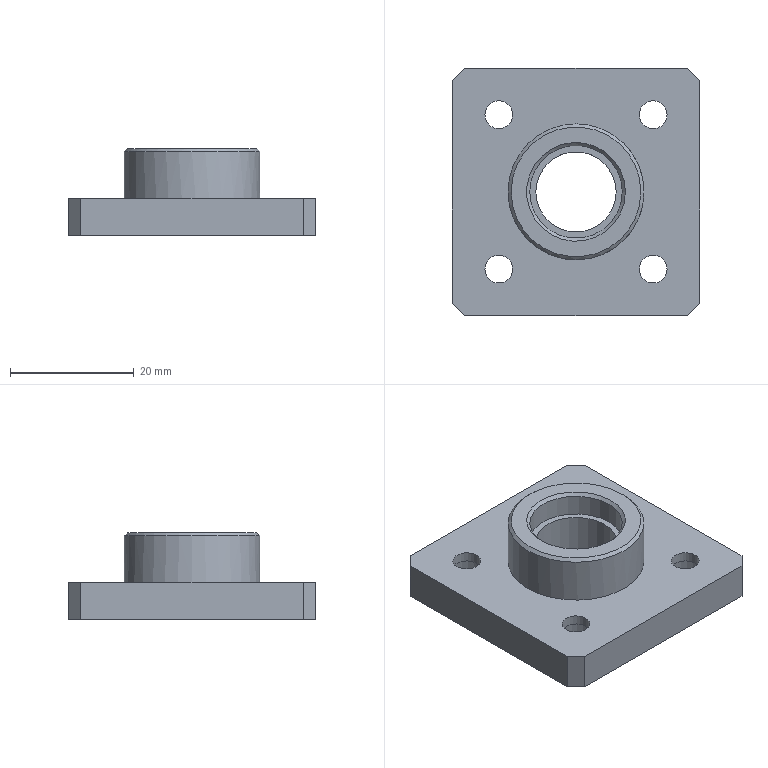Part | NX | 1 solid | 29 faces | box 40 x 40 x 14 mm | volume 9558 mm3 | plane 16 | cylinder 11 | cone 2 | commonest cylinder face diameters 4.5 x4 8 x4 13 x1 15 x1 22 x1
STEP:
#1=CARTESIAN_POINT('',(10.25,12.5,6.));
#2=VERTEX_POINT('',#1);
#3=CARTESIAN_POINT('',(12.5,12.5,6.));
#4=DIRECTION('',(0.,0.,-1.));
#5=DIRECTION('',(-1.,0.,0.));
#6=AXIS2_PLACEMENT_3D('',#3,#4,#5);
#7=CIRCLE('',#6,2.25);
#8=EDGE_CURVE('',#2,#2,#7,.T.);
#9=ORIENTED_EDGE('',*,*,#8,.T.);
#10=EDGE_LOOP('',(#9));
#11=FACE_BOUND('',#10,.T.);
#12=CARTESIAN_POINT('',(10.25,-12.5,6.));
#13=VERTEX_POINT('',#12);
#14=CARTESIAN_POINT('',(12.5,-12.5,6.));
#15=DIRECTION('',(0.,0.,-1.));
#16=DIRECTION('',(-1.,0.,0.));
#17=AXIS2_PLACEMENT_3D('',#14,#15,#16);
#18=CIRCLE('',#17,2.25);
#19=EDGE_CURVE('',#13,#13,#18,.T.);
#20=ORIENTED_EDGE('',*,*,#19,.T.);
#21=EDGE_LOOP('',(#20));
#22=FACE_BOUND('',#21,.T.);
#23=CARTESIAN_POINT('',(-14.75,12.5,6.));
#24=VERTEX_POINT('',#23);
#25=CARTESIAN_POINT('',(-12.5,12.5,6.));
#26=DIRECTION('',(0.,0.,-1.));
#27=DIRECTION('',(-1.,0.,0.));
#28=AXIS2_PLACEMENT_3D('',#25,#26,#27);
#29=CIRCLE('',#28,2.25);
#30=EDGE_CURVE('',#24,#24,#29,.T.);
#31=ORIENTED_EDGE('',*,*,#30,.T.);
#32=EDGE_LOOP('',(#31));
#33=FACE_BOUND('',#32,.T.);
#34=CARTESIAN_POINT('',(-14.75,-12.5,6.));
#35=VERTEX_POINT('',#34);
#36=CARTESIAN_POINT('',(-12.5,-12.5,6.));
#37=DIRECTION('',(0.,0.,-1.));
#38=DIRECTION('',(-1.,0.,0.));
#39=AXIS2_PLACEMENT_3D('',#36,#37,#38);
#40=CIRCLE('',#39,2.25);
#41=EDGE_CURVE('',#35,#35,#40,.T.);
#42=ORIENTED_EDGE('',*,*,#41,.T.);
#43=EDGE_LOOP('',(#42));
#44=FACE_BOUND('',#43,.T.);
#45=CARTESIAN_POINT('',(-18.,-20.,6.));
#46=VERTEX_POINT('',#45);
#47=CARTESIAN_POINT('',(18.,-20.,6.));
#48=VERTEX_POINT('',#47);
#49=CARTESIAN_POINT('',(-20.,-20.,6.));
#50=DIRECTION('',(1.,0.,0.));
#51=VECTOR('',#50,1000.);
#52=LINE('',#49,#51);
#53=EDGE_CURVE('',#46,#48,#52,.T.);
#54=ORIENTED_EDGE('',*,*,#53,.T.);
#55=CARTESIAN_POINT('',(20.,-18.,6.));
#56=VERTEX_POINT('',#55);
#57=CARTESIAN_POINT('',(20.,-18.,6.));
#58=DIRECTION('',(-0.7071,-0.7071,0.));
#59=VECTOR('',#58,1000.);
#60=LINE('',#57,#59);
#61=EDGE_CURVE('',#48,#56,#60,.F.);
#62=ORIENTED_EDGE('',*,*,#61,.T.);
#63=CARTESIAN_POINT('',(20.,18.,6.));
#64=VERTEX_POINT('',#63);
#65=CARTESIAN_POINT('',(20.,-20.,6.));
#66=DIRECTION('',(0.,1.,0.));
#67=VECTOR('',#66,1000.);
#68=LINE('',#65,#67);
#69=EDGE_CURVE('',#56,#64,#68,.T.);
#70=ORIENTED_EDGE('',*,*,#69,.T.);
#71=CARTESIAN_POINT('',(18.,20.,6.));
#72=VERTEX_POINT('',#71);
#73=CARTESIAN_POINT('',(18.,20.,6.));
#74=DIRECTION('',(0.7071,-0.7071,0.));
#75=VECTOR('',#74,1000.);
#76=LINE('',#73,#75);
#77=EDGE_CURVE('',#64,#72,#76,.F.);
#78=ORIENTED_EDGE('',*,*,#77,.T.);
#79=CARTESIAN_POINT('',(-18.,20.,6.));
#80=VERTEX_POINT('',#79);
#81=CARTESIAN_POINT('',(-20.,20.,6.));
#82=DIRECTION('',(-1.,0.,0.));
#83=VECTOR('',#82,1000.);
#84=LINE('',#81,#83);
#85=EDGE_CURVE('',#72,#80,#84,.T.);
#86=ORIENTED_EDGE('',*,*,#85,.T.);
#87=CARTESIAN_POINT('',(-20.,18.,6.));
#88=VERTEX_POINT('',#87);
#89=CARTESIAN_POINT('',(-20.,18.,6.));
#90=DIRECTION('',(0.7071,0.7071,0.));
#91=VECTOR('',#90,1000.);
#92=LINE('',#89,#91);
#93=EDGE_CURVE('',#80,#88,#92,.F.);
#94=ORIENTED_EDGE('',*,*,#93,.T.);
#95=CARTESIAN_POINT('',(-20.,-18.,6.));
#96=VERTEX_POINT('',#95);
#97=CARTESIAN_POINT('',(-20.,-20.,6.));
#98=DIRECTION('',(0.,-1.,0.));
#99=VECTOR('',#98,1000.);
#100=LINE('',#97,#99);
#101=EDGE_CURVE('',#88,#96,#100,.T.);
#102=ORIENTED_EDGE('',*,*,#101,.T.);
#103=CARTESIAN_POINT('',(-18.,-20.,6.));
#104=DIRECTION('',(-0.7071,0.7071,0.));
#105=VECTOR('',#104,1000.);
#106=LINE('',#103,#105);
#107=EDGE_CURVE('',#96,#46,#106,.F.);
#108=ORIENTED_EDGE('',*,*,#107,.T.);
#109=EDGE_LOOP('',(#54,#62,#70,#78,#86,#94,#102,#108));
#110=FACE_BOUND('',#109,.T.);
#111=CARTESIAN_POINT('',(-11.,0.,6.));
#112=VERTEX_POINT('',#111);
#113=CARTESIAN_POINT('',(0.,0.,6.));
#114=DIRECTION('',(0.,0.,-1.));
#115=DIRECTION('',(-1.,0.,0.));
#116=AXIS2_PLACEMENT_3D('',#113,#114,#115);
#117=CIRCLE('',#116,11.);
#118=EDGE_CURVE('',#112,#112,#117,.F.);
#119=ORIENTED_EDGE('',*,*,#118,.F.);
#120=EDGE_LOOP('',(#119));
#121=FACE_BOUND('',#120,.T.);
#122=CARTESIAN_POINT('',(0.,0.,6.));
#123=DIRECTION('',(0.,0.,-1.));
#124=DIRECTION('',(-1.,0.,0.));
#125=AXIS2_PLACEMENT_3D('',#122,#123,#124);
#126=PLANE('',#125);
#127=ADVANCED_FACE('',(#11,#22,#33,#44,#110,#121),#126,.F.);
#128=ORIENTED_EDGE('',*,*,#69,.F.);
#129=CARTESIAN_POINT('',(20.,-18.,0.));
#130=VERTEX_POINT('',#129);
#131=CARTESIAN_POINT('',(20.,-18.,6.));
#132=DIRECTION('',(0.,0.,-1.));
#133=VECTOR('',#132,1000.);
#134=LINE('',#131,#133);
#135=EDGE_CURVE('',#56,#130,#134,.T.);
#136=ORIENTED_EDGE('',*,*,#135,.T.);
#137=CARTESIAN_POINT('',(20.,18.,0.));
#138=VERTEX_POINT('',#137);
#139=CARTESIAN_POINT('',(20.,-20.,0.));
#140=DIRECTION('',(0.,1.,0.));
#141=VECTOR('',#140,1000.);
#142=LINE('',#139,#141);
#143=EDGE_CURVE('',#130,#138,#142,.T.);
#144=ORIENTED_EDGE('',*,*,#143,.T.);
#145=CARTESIAN_POINT('',(20.,18.,6.));
#146=DIRECTION('',(0.,0.,1.));
#147=VECTOR('',#146,1000.);
#148=LINE('',#145,#147);
#149=EDGE_CURVE('',#138,#64,#148,.T.);
#150=ORIENTED_EDGE('',*,*,#149,.T.);
#151=EDGE_LOOP('',(#128,#136,#144,#150));
#152=FACE_BOUND('',#151,.T.);
#153=CARTESIAN_POINT('',(20.,-20.,6.));
#154=DIRECTION('',(-1.,0.,0.));
#155=DIRECTION('',(0.,0.,1.));
#156=AXIS2_PLACEMENT_3D('',#153,#154,#155);
#157=PLANE('',#156);
#158=ADVANCED_FACE('',(#152),#157,.F.);
#159=CARTESIAN_POINT('',(18.,20.,0.));
#160=VERTEX_POINT('',#159);
#161=CARTESIAN_POINT('',(-18.,20.,0.));
#162=VERTEX_POINT('',#161);
#163=CARTESIAN_POINT('',(-20.,20.,0.));
#164=DIRECTION('',(-1.,0.,0.));
#165=VECTOR('',#164,1000.);
#166=LINE('',#163,#165);
#167=EDGE_CURVE('',#160,#162,#166,.T.);
#168=ORIENTED_EDGE('',*,*,#167,.T.);
#169=CARTESIAN_POINT('',(-18.,20.,6.));
#170=DIRECTION('',(0.,0.,1.));
#171=VECTOR('',#170,1000.);
#172=LINE('',#169,#171);
#173=EDGE_CURVE('',#162,#80,#172,.T.);
#174=ORIENTED_EDGE('',*,*,#173,.T.);
#175=ORIENTED_EDGE('',*,*,#85,.F.);
#176=CARTESIAN_POINT('',(18.,20.,6.));
#177=DIRECTION('',(0.,0.,-1.));
#178=VECTOR('',#177,1000.);
#179=LINE('',#176,#178);
#180=EDGE_CURVE('',#72,#160,#179,.T.);
#181=ORIENTED_EDGE('',*,*,#180,.T.);
#182=EDGE_LOOP('',(#168,#174,#175,#181));
#183=FACE_BOUND('',#182,.T.);
#184=CARTESIAN_POINT('',(-20.,20.,6.));
#185=DIRECTION('',(0.,-1.,0.));
#186=DIRECTION('',(0.,0.,-1.));
#187=AXIS2_PLACEMENT_3D('',#184,#185,#186);
#188=PLANE('',#187);
#189=ADVANCED_FACE('',(#183),#188,.F.);
#190=CARTESIAN_POINT('',(-20.,18.,0.));
#191=VERTEX_POINT('',#190);
#192=CARTESIAN_POINT('',(-20.,-18.,0.));
#193=VERTEX_POINT('',#192);
#194=CARTESIAN_POINT('',(-20.,-20.,0.));
#195=DIRECTION('',(0.,-1.,0.));
#196=VECTOR('',#195,1000.);
#197=LINE('',#194,#196);
#198=EDGE_CURVE('',#191,#193,#197,.T.);
#199=ORIENTED_EDGE('',*,*,#198,.T.);
#200=CARTESIAN_POINT('',(-20.,-18.,6.));
#201=DIRECTION('',(0.,0.,1.));
#202=VECTOR('',#201,1000.);
#203=LINE('',#200,#202);
#204=EDGE_CURVE('',#193,#96,#203,.T.);
#205=ORIENTED_EDGE('',*,*,#204,.T.);
#206=ORIENTED_EDGE('',*,*,#101,.F.);
#207=CARTESIAN_POINT('',(-20.,18.,6.));
#208=DIRECTION('',(0.,0.,-1.));
#209=VECTOR('',#208,1000.);
#210=LINE('',#207,#209);
#211=EDGE_CURVE('',#88,#191,#210,.T.);
#212=ORIENTED_EDGE('',*,*,#211,.T.);
#213=EDGE_LOOP('',(#199,#205,#206,#212));
#214=FACE_BOUND('',#213,.T.);
#215=CARTESIAN_POINT('',(-20.,-20.,6.));
#216=DIRECTION('',(1.,0.,0.));
#217=DIRECTION('',(0.,0.,-1.));
#218=AXIS2_PLACEMENT_3D('',#215,#216,#217);
#219=PLANE('',#218);
#220=ADVANCED_FACE('',(#214),#219,.F.);
#221=CARTESIAN_POINT('',(-18.,-20.,0.));
#222=VERTEX_POINT('',#221);
#223=CARTESIAN_POINT('',(18.,-20.,0.));
#224=VERTEX_POINT('',#223);
#225=CARTESIAN_POINT('',(-20.,-20.,0.));
#226=DIRECTION('',(1.,0.,0.));
#227=VECTOR('',#226,1000.);
#228=LINE('',#225,#227);
#229=EDGE_CURVE('',#222,#224,#228,.T.);
#230=ORIENTED_EDGE('',*,*,#229,.T.);
#231=CARTESIAN_POINT('',(18.,-20.,6.));
#232=DIRECTION('',(0.,0.,1.));
#233=VECTOR('',#232,1000.);
#234=LINE('',#231,#233);
#235=EDGE_CURVE('',#224,#48,#234,.T.);
#236=ORIENTED_EDGE('',*,*,#235,.T.);
#237=ORIENTED_EDGE('',*,*,#53,.F.);
#238=CARTESIAN_POINT('',(-18.,-20.,6.));
#239=DIRECTION('',(0.,0.,-1.));
#240=VECTOR('',#239,1000.);
#241=LINE('',#238,#240);
#242=EDGE_CURVE('',#46,#222,#241,.T.);
#243=ORIENTED_EDGE('',*,*,#242,.T.);
#244=EDGE_LOOP('',(#230,#236,#237,#243));
#245=FACE_BOUND('',#244,.T.);
#246=CARTESIAN_POINT('',(-20.,-20.,6.));
#247=DIRECTION('',(0.,1.,0.));
#248=DIRECTION('',(0.,0.,1.));
#249=AXIS2_PLACEMENT_3D('',#246,#247,#248);
#250=PLANE('',#249);
#251=ADVANCED_FACE('',(#245),#250,.F.);
#252=CARTESIAN_POINT('',(8.5,12.5,0.));
#253=VERTEX_POINT('',#252);
#254=CARTESIAN_POINT('',(12.5,12.5,0.));
#255=DIRECTION('',(0.,0.,-1.));
#256=DIRECTION('',(-1.,0.,0.));
#257=AXIS2_PLACEMENT_3D('',#254,#255,#256);
#258=CIRCLE('',#257,4.);
#259=EDGE_CURVE('',#253,#253,#258,.T.);
#260=ORIENTED_EDGE('',*,*,#259,.F.);
#261=EDGE_LOOP('',(#260));
#262=FACE_BOUND('',#261,.T.);
#263=CARTESIAN_POINT('',(8.5,-12.5,0.));
#264=VERTEX_POINT('',#263);
#265=CARTESIAN_POINT('',(12.5,-12.5,0.));
#266=DIRECTION('',(0.,0.,-1.));
#267=DIRECTION('',(-1.,0.,0.));
#268=AXIS2_PLACEMENT_3D('',#265,#266,#267);
#269=CIRCLE('',#268,4.);
#270=EDGE_CURVE('',#264,#264,#269,.T.);
#271=ORIENTED_EDGE('',*,*,#270,.F.);
#272=EDGE_LOOP('',(#271));
#273=FACE_BOUND('',#272,.T.);
#274=CARTESIAN_POINT('',(-16.5,12.5,0.));
#275=VERTEX_POINT('',#274);
#276=CARTESIAN_POINT('',(-12.5,12.5,0.));
#277=DIRECTION('',(0.,0.,-1.));
#278=DIRECTION('',(-1.,0.,0.));
#279=AXIS2_PLACEMENT_3D('',#276,#277,#278);
#280=CIRCLE('',#279,4.);
#281=EDGE_CURVE('',#275,#275,#280,.T.);
#282=ORIENTED_EDGE('',*,*,#281,.F.);
#283=EDGE_LOOP('',(#282));
#284=FACE_BOUND('',#283,.T.);
#285=CARTESIAN_POINT('',(-16.5,-12.5,0.));
#286=VERTEX_POINT('',#285);
#287=CARTESIAN_POINT('',(-12.5,-12.5,0.));
#288=DIRECTION('',(0.,0.,-1.));
#289=DIRECTION('',(-1.,0.,0.));
#290=AXIS2_PLACEMENT_3D('',#287,#288,#289);
#291=CIRCLE('',#290,4.);
#292=EDGE_CURVE('',#286,#286,#291,.T.);
#293=ORIENTED_EDGE('',*,*,#292,.F.);
#294=EDGE_LOOP('',(#293));
#295=FACE_BOUND('',#294,.T.);
#296=CARTESIAN_POINT('',(-6.5,0.,0.));
#297=VERTEX_POINT('',#296);
#298=CARTESIAN_POINT('',(0.,0.,0.));
#299=DIRECTION('',(0.,0.,-1.));
#300=DIRECTION('',(-1.,0.,0.));
#301=AXIS2_PLACEMENT_3D('',#298,#299,#300);
#302=CIRCLE('',#301,6.5);
#303=EDGE_CURVE('',#297,#297,#302,.T.);
#304=ORIENTED_EDGE('',*,*,#303,.F.);
#305=EDGE_LOOP('',(#304));
#306=FACE_BOUND('',#305,.T.);
#307=ORIENTED_EDGE('',*,*,#143,.F.);
#308=CARTESIAN_POINT('',(19.,-19.,0.));
#309=DIRECTION('',(0.7071,0.7071,0.));
#310=VECTOR('',#309,1000.);
#311=LINE('',#308,#310);
#312=EDGE_CURVE('',#130,#224,#311,.F.);
#313=ORIENTED_EDGE('',*,*,#312,.T.);
#314=ORIENTED_EDGE('',*,*,#229,.F.);
#315=CARTESIAN_POINT('',(-19.,-19.,0.));
#316=DIRECTION('',(0.7071,-0.7071,0.));
#317=VECTOR('',#316,1000.);
#318=LINE('',#315,#317);
#319=EDGE_CURVE('',#222,#193,#318,.F.);
#320=ORIENTED_EDGE('',*,*,#319,.T.);
#321=ORIENTED_EDGE('',*,*,#198,.F.);
#322=CARTESIAN_POINT('',(-19.,19.,0.));
#323=DIRECTION('',(-0.7071,-0.7071,0.));
#324=VECTOR('',#323,1000.);
#325=LINE('',#322,#324);
#326=EDGE_CURVE('',#191,#162,#325,.F.);
#327=ORIENTED_EDGE('',*,*,#326,.T.);
#328=ORIENTED_EDGE('',*,*,#167,.F.);
#329=CARTESIAN_POINT('',(19.,19.,0.));
#330=DIRECTION('',(-0.7071,0.7071,0.));
#331=VECTOR('',#330,1000.);
#332=LINE('',#329,#331);
#333=EDGE_CURVE('',#160,#138,#332,.F.);
#334=ORIENTED_EDGE('',*,*,#333,.T.);
#335=EDGE_LOOP('',(#307,#313,#314,#320,#321,#327,#328,#334));
#336=FACE_BOUND('',#335,.T.);
#337=CARTESIAN_POINT('',(0.,0.,0.));
#338=DIRECTION('',(0.,0.,-1.));
#339=DIRECTION('',(-1.,0.,0.));
#340=AXIS2_PLACEMENT_3D('',#337,#338,#339);
#341=PLANE('',#340);
#342=ADVANCED_FACE('',(#262,#273,#284,#295,#306,#336),#341,.T.);
#343=CARTESIAN_POINT('',(11.,0.,13.5));
#344=VERTEX_POINT('',#343);
#345=CARTESIAN_POINT('',(0.,0.,13.5));
#346=DIRECTION('',(0.,0.,1.));
#347=DIRECTION('',(1.,0.,0.));
#348=AXIS2_PLACEMENT_3D('',#345,#346,#347);
#349=CIRCLE('',#348,11.);
#350=EDGE_CURVE('',#344,#344,#349,.F.);
#351=ORIENTED_EDGE('',*,*,#350,.T.);
#352=EDGE_LOOP('',(#351));
#353=FACE_BOUND('',#352,.T.);
#354=ORIENTED_EDGE('',*,*,#118,.T.);
#355=EDGE_LOOP('',(#354));
#356=FACE_BOUND('',#355,.T.);
#357=CARTESIAN_POINT('',(0.,0.,14.));
#358=DIRECTION('',(0.,0.,-1.));
#359=DIRECTION('',(-1.,0.,0.));
#360=AXIS2_PLACEMENT_3D('',#357,#358,#359);
#361=CYLINDRICAL_SURFACE('',#360,11.);
#362=ADVANCED_FACE('',(#353,#356),#361,.T.);
#363=CARTESIAN_POINT('',(8.,0.,14.));
#364=VERTEX_POINT('',#363);
#365=CARTESIAN_POINT('',(0.,0.,14.));
#366=DIRECTION('',(0.,0.,1.));
#367=DIRECTION('',(1.,0.,0.));
#368=AXIS2_PLACEMENT_3D('',#365,#366,#367);
#369=CIRCLE('',#368,8.);
#370=EDGE_CURVE('',#364,#364,#369,.F.);
#371=ORIENTED_EDGE('',*,*,#370,.T.);
#372=EDGE_LOOP('',(#371));
#373=FACE_BOUND('',#372,.T.);
#374=CARTESIAN_POINT('',(10.5,0.,14.));
#375=VERTEX_POINT('',#374);
#376=CARTESIAN_POINT('',(0.,0.,14.));
#377=DIRECTION('',(0.,0.,1.));
#378=DIRECTION('',(1.,0.,0.));
#379=AXIS2_PLACEMENT_3D('',#376,#377,#378);
#380=CIRCLE('',#379,10.5);
#381=EDGE_CURVE('',#375,#375,#380,.T.);
#382=ORIENTED_EDGE('',*,*,#381,.T.);
#383=EDGE_LOOP('',(#382));
#384=FACE_BOUND('',#383,.T.);
#385=CARTESIAN_POINT('',(0.,0.,14.));
#386=DIRECTION('',(0.,0.,1.));
#387=DIRECTION('',(1.,0.,0.));
#388=AXIS2_PLACEMENT_3D('',#385,#386,#387);
#389=PLANE('',#388);
#390=ADVANCED_FACE('',(#373,#384),#389,.T.);
#391=CARTESIAN_POINT('',(7.5,0.,13.5));
#392=VERTEX_POINT('',#391);
#393=CARTESIAN_POINT('',(0.,0.,13.5));
#394=DIRECTION('',(0.,0.,1.));
#395=DIRECTION('',(1.,0.,0.));
#396=AXIS2_PLACEMENT_3D('',#393,#394,#395);
#397=CIRCLE('',#396,7.5);
#398=EDGE_CURVE('',#392,#392,#397,.T.);
#399=ORIENTED_EDGE('',*,*,#398,.T.);
#400=EDGE_LOOP('',(#399));
#401=FACE_BOUND('',#400,.T.);
#402=CARTESIAN_POINT('',(7.5,0.,10.));
#403=VERTEX_POINT('',#402);
#404=CARTESIAN_POINT('',(0.,0.,10.));
#405=DIRECTION('',(0.,0.,1.));
#406=DIRECTION('',(1.,0.,0.));
#407=AXIS2_PLACEMENT_3D('',#404,#405,#406);
#408=CIRCLE('',#407,7.5);
#409=EDGE_CURVE('',#403,#403,#408,.T.);
#410=ORIENTED_EDGE('',*,*,#409,.F.);
#411=EDGE_LOOP('',(#410));
#412=FACE_BOUND('',#411,.T.);
#413=CARTESIAN_POINT('',(0.,0.,10.));
#414=DIRECTION('',(0.,0.,1.));
#415=DIRECTION('',(1.,0.,0.));
#416=AXIS2_PLACEMENT_3D('',#413,#414,#415);
#417=CYLINDRICAL_SURFACE('',#416,7.5);
#418=ADVANCED_FACE('',(#401,#412),#417,.F.);
#419=CARTESIAN_POINT('',(6.5,0.,10.));
#420=VERTEX_POINT('',#419);
#421=CARTESIAN_POINT('',(0.,0.,10.));
#422=DIRECTION('',(0.,0.,1.));
#423=DIRECTION('',(1.,0.,0.));
#424=AXIS2_PLACEMENT_3D('',#421,#422,#423);
#425=CIRCLE('',#424,6.5);
#426=EDGE_CURVE('',#420,#420,#425,.T.);
#427=ORIENTED_EDGE('',*,*,#426,.F.);
#428=EDGE_LOOP('',(#427));
#429=FACE_BOUND('',#428,.T.);
#430=ORIENTED_EDGE('',*,*,#409,.T.);
#431=EDGE_LOOP('',(#430));
#432=FACE_BOUND('',#431,.T.);
#433=CARTESIAN_POINT('',(0.,0.,10.));
#434=DIRECTION('',(0.,0.,1.));
#435=DIRECTION('',(1.,0.,0.));
#436=AXIS2_PLACEMENT_3D('',#433,#434,#435);
#437=PLANE('',#436);
#438=ADVANCED_FACE('',(#429,#432),#437,.T.);
#439=ORIENTED_EDGE('',*,*,#426,.T.);
#440=EDGE_LOOP('',(#439));
#441=FACE_BOUND('',#440,.T.);
#442=ORIENTED_EDGE('',*,*,#303,.T.);
#443=EDGE_LOOP('',(#442));
#444=FACE_BOUND('',#443,.T.);
#445=CARTESIAN_POINT('',(0.,0.,14.));
#446=DIRECTION('',(0.,0.,-1.));
#447=DIRECTION('',(-1.,0.,0.));
#448=AXIS2_PLACEMENT_3D('',#445,#446,#447);
#449=CYLINDRICAL_SURFACE('',#448,6.5);
#450=ADVANCED_FACE('',(#441,#444),#449,.F.);
#451=ORIENTED_EDGE('',*,*,#61,.F.);
#452=ORIENTED_EDGE('',*,*,#235,.F.);
#453=ORIENTED_EDGE('',*,*,#312,.F.);
#454=ORIENTED_EDGE('',*,*,#135,.F.);
#455=EDGE_LOOP('',(#451,#452,#453,#454));
#456=FACE_BOUND('',#455,.T.);
#457=CARTESIAN_POINT('',(20.,-18.,6.));
#458=DIRECTION('',(-0.7071,0.7071,0.));
#459=DIRECTION('',(0.,0.,-1.));
#460=AXIS2_PLACEMENT_3D('',#457,#458,#459);
#461=PLANE('',#460);
#462=ADVANCED_FACE('',(#456),#461,.F.);
#463=ORIENTED_EDGE('',*,*,#107,.F.);
#464=ORIENTED_EDGE('',*,*,#204,.F.);
#465=ORIENTED_EDGE('',*,*,#319,.F.);
#466=ORIENTED_EDGE('',*,*,#242,.F.);
#467=EDGE_LOOP('',(#463,#464,#465,#466));
#468=FACE_BOUND('',#467,.T.);
#469=CARTESIAN_POINT('',(-18.,-20.,6.));
#470=DIRECTION('',(0.7071,0.7071,0.));
#471=DIRECTION('',(0.,0.,-1.));
#472=AXIS2_PLACEMENT_3D('',#469,#470,#471);
#473=PLANE('',#472);
#474=ADVANCED_FACE('',(#468),#473,.F.);
#475=ORIENTED_EDGE('',*,*,#93,.F.);
#476=ORIENTED_EDGE('',*,*,#173,.F.);
#477=ORIENTED_EDGE('',*,*,#326,.F.);
#478=ORIENTED_EDGE('',*,*,#211,.F.);
#479=EDGE_LOOP('',(#475,#476,#477,#478));
#480=FACE_BOUND('',#479,.T.);
#481=CARTESIAN_POINT('',(-20.,18.,6.));
#482=DIRECTION('',(0.7071,-0.7071,0.));
#483=DIRECTION('',(0.,0.,-1.));
#484=AXIS2_PLACEMENT_3D('',#481,#482,#483);
#485=PLANE('',#484);
#486=ADVANCED_FACE('',(#480),#485,.F.);
#487=ORIENTED_EDGE('',*,*,#77,.F.);
#488=ORIENTED_EDGE('',*,*,#149,.F.);
#489=ORIENTED_EDGE('',*,*,#333,.F.);
#490=ORIENTED_EDGE('',*,*,#180,.F.);
#491=EDGE_LOOP('',(#487,#488,#489,#490));
#492=FACE_BOUND('',#491,.T.);
#493=CARTESIAN_POINT('',(18.,20.,6.));
#494=DIRECTION('',(-0.7071,-0.7071,0.));
#495=DIRECTION('',(0.,0.,-1.));
#496=AXIS2_PLACEMENT_3D('',#493,#494,#495);
#497=PLANE('',#496);
#498=ADVANCED_FACE('',(#492),#497,.F.);
#499=CARTESIAN_POINT('',(-14.75,-12.5,4.4));
#500=VERTEX_POINT('',#499);
#501=CARTESIAN_POINT('',(-12.5,-12.5,4.4));
#502=DIRECTION('',(0.,0.,-1.));
#503=DIRECTION('',(-1.,0.,0.));
#504=AXIS2_PLACEMENT_3D('',#501,#502,#503);
#505=CIRCLE('',#504,2.25);
#506=EDGE_CURVE('',#500,#500,#505,.T.);
#507=ORIENTED_EDGE('',*,*,#506,.T.);
#508=EDGE_LOOP('',(#507));
#509=FACE_BOUND('',#508,.T.);
#510=ORIENTED_EDGE('',*,*,#41,.F.);
#511=EDGE_LOOP('',(#510));
#512=FACE_BOUND('',#511,.T.);
#513=CARTESIAN_POINT('',(-12.5,-12.5,0.));
#514=DIRECTION('',(0.,0.,-1.));
#515=DIRECTION('',(-1.,0.,0.));
#516=AXIS2_PLACEMENT_3D('',#513,#514,#515);
#517=CYLINDRICAL_SURFACE('',#516,2.25);
#518=ADVANCED_FACE('',(#509,#512),#517,.F.);
#519=ORIENTED_EDGE('',*,*,#506,.F.);
#520=EDGE_LOOP('',(#519));
#521=FACE_BOUND('',#520,.T.);
#522=CARTESIAN_POINT('',(-16.5,-12.5,4.4));
#523=VERTEX_POINT('',#522);
#524=CARTESIAN_POINT('',(-12.5,-12.5,4.4));
#525=DIRECTION('',(0.,0.,-1.));
#526=DIRECTION('',(-1.,0.,0.));
#527=AXIS2_PLACEMENT_3D('',#524,#525,#526);
#528=CIRCLE('',#527,4.);
#529=EDGE_CURVE('',#523,#523,#528,.T.);
#530=ORIENTED_EDGE('',*,*,#529,.T.);
#531=EDGE_LOOP('',(#530));
#532=FACE_BOUND('',#531,.T.);
#533=CARTESIAN_POINT('',(-10.25,-12.5,4.4));
#534=DIRECTION('',(0.,0.,1.));
#535=DIRECTION('',(1.,0.,0.));
#536=AXIS2_PLACEMENT_3D('',#533,#534,#535);
#537=PLANE('',#536);
#538=ADVANCED_FACE('',(#521,#532),#537,.F.);
#539=ORIENTED_EDGE('',*,*,#529,.F.);
#540=EDGE_LOOP('',(#539));
#541=FACE_BOUND('',#540,.T.);
#542=ORIENTED_EDGE('',*,*,#292,.T.);
#543=EDGE_LOOP('',(#542));
#544=FACE_BOUND('',#543,.T.);
#545=CARTESIAN_POINT('',(-12.5,-12.5,0.));
#546=DIRECTION('',(0.,0.,-1.));
#547=DIRECTION('',(-1.,0.,0.));
#548=AXIS2_PLACEMENT_3D('',#545,#546,#547);
#549=CYLINDRICAL_SURFACE('',#548,4.);
#550=ADVANCED_FACE('',(#541,#544),#549,.F.);
#551=CARTESIAN_POINT('',(-14.75,12.5,4.4));
#552=VERTEX_POINT('',#551);
#553=CARTESIAN_POINT('',(-12.5,12.5,4.4));
#554=DIRECTION('',(0.,0.,-1.));
#555=DIRECTION('',(-1.,0.,0.));
#556=AXIS2_PLACEMENT_3D('',#553,#554,#555);
#557=CIRCLE('',#556,2.25);
#558=EDGE_CURVE('',#552,#552,#557,.T.);
#559=ORIENTED_EDGE('',*,*,#558,.T.);
#560=EDGE_LOOP('',(#559));
#561=FACE_BOUND('',#560,.T.);
#562=ORIENTED_EDGE('',*,*,#30,.F.);
#563=EDGE_LOOP('',(#562));
#564=FACE_BOUND('',#563,.T.);
#565=CARTESIAN_POINT('',(-12.5,12.5,0.));
#566=DIRECTION('',(0.,0.,-1.));
#567=DIRECTION('',(-1.,0.,0.));
#568=AXIS2_PLACEMENT_3D('',#565,#566,#567);
#569=CYLINDRICAL_SURFACE('',#568,2.25);
#570=ADVANCED_FACE('',(#561,#564),#569,.F.);
#571=ORIENTED_EDGE('',*,*,#558,.F.);
#572=EDGE_LOOP('',(#571));
#573=FACE_BOUND('',#572,.T.);
#574=CARTESIAN_POINT('',(-16.5,12.5,4.4));
#575=VERTEX_POINT('',#574);
#576=CARTESIAN_POINT('',(-12.5,12.5,4.4));
#577=DIRECTION('',(0.,0.,-1.));
#578=DIRECTION('',(-1.,0.,0.));
#579=AXIS2_PLACEMENT_3D('',#576,#577,#578);
#580=CIRCLE('',#579,4.);
#581=EDGE_CURVE('',#575,#575,#580,.T.);
#582=ORIENTED_EDGE('',*,*,#581,.T.);
#583=EDGE_LOOP('',(#582));
#584=FACE_BOUND('',#583,.T.);
#585=CARTESIAN_POINT('',(-10.25,12.5,4.4));
#586=DIRECTION('',(0.,0.,1.));
#587=DIRECTION('',(1.,0.,0.));
#588=AXIS2_PLACEMENT_3D('',#585,#586,#587);
#589=PLANE('',#588);
#590=ADVANCED_FACE('',(#573,#584),#589,.F.);
#591=ORIENTED_EDGE('',*,*,#581,.F.);
#592=EDGE_LOOP('',(#591));
#593=FACE_BOUND('',#592,.T.);
#594=ORIENTED_EDGE('',*,*,#281,.T.);
#595=EDGE_LOOP('',(#594));
#596=FACE_BOUND('',#595,.T.);
#597=CARTESIAN_POINT('',(-12.5,12.5,0.));
#598=DIRECTION('',(0.,0.,-1.));
#599=DIRECTION('',(-1.,0.,0.));
#600=AXIS2_PLACEMENT_3D('',#597,#598,#599);
#601=CYLINDRICAL_SURFACE('',#600,4.);
#602=ADVANCED_FACE('',(#593,#596),#601,.F.);
#603=CARTESIAN_POINT('',(10.25,-12.5,4.4));
#604=VERTEX_POINT('',#603);
#605=CARTESIAN_POINT('',(12.5,-12.5,4.4));
#606=DIRECTION('',(0.,0.,-1.));
#607=DIRECTION('',(-1.,0.,0.));
#608=AXIS2_PLACEMENT_3D('',#605,#606,#607);
#609=CIRCLE('',#608,2.25);
#610=EDGE_CURVE('',#604,#604,#609,.T.);
#611=ORIENTED_EDGE('',*,*,#610,.T.);
#612=EDGE_LOOP('',(#611));
#613=FACE_BOUND('',#612,.T.);
#614=ORIENTED_EDGE('',*,*,#19,.F.);
#615=EDGE_LOOP('',(#614));
#616=FACE_BOUND('',#615,.T.);
#617=CARTESIAN_POINT('',(12.5,-12.5,0.));
#618=DIRECTION('',(0.,0.,-1.));
#619=DIRECTION('',(-1.,0.,0.));
#620=AXIS2_PLACEMENT_3D('',#617,#618,#619);
#621=CYLINDRICAL_SURFACE('',#620,2.25);
#622=ADVANCED_FACE('',(#613,#616),#621,.F.);
#623=ORIENTED_EDGE('',*,*,#610,.F.);
#624=EDGE_LOOP('',(#623));
#625=FACE_BOUND('',#624,.T.);
#626=CARTESIAN_POINT('',(8.5,-12.5,4.4));
#627=VERTEX_POINT('',#626);
#628=CARTESIAN_POINT('',(12.5,-12.5,4.4));
#629=DIRECTION('',(0.,0.,-1.));
#630=DIRECTION('',(-1.,0.,0.));
#631=AXIS2_PLACEMENT_3D('',#628,#629,#630);
#632=CIRCLE('',#631,4.);
#633=EDGE_CURVE('',#627,#627,#632,.T.);
#634=ORIENTED_EDGE('',*,*,#633,.T.);
#635=EDGE_LOOP('',(#634));
#636=FACE_BOUND('',#635,.T.);
#637=CARTESIAN_POINT('',(14.75,-12.5,4.4));
#638=DIRECTION('',(0.,0.,1.));
#639=DIRECTION('',(1.,0.,0.));
#640=AXIS2_PLACEMENT_3D('',#637,#638,#639);
#641=PLANE('',#640);
#642=ADVANCED_FACE('',(#625,#636),#641,.F.);
#643=ORIENTED_EDGE('',*,*,#633,.F.);
#644=EDGE_LOOP('',(#643));
#645=FACE_BOUND('',#644,.T.);
#646=ORIENTED_EDGE('',*,*,#270,.T.);
#647=EDGE_LOOP('',(#646));
#648=FACE_BOUND('',#647,.T.);
#649=CARTESIAN_POINT('',(12.5,-12.5,0.));
#650=DIRECTION('',(0.,0.,-1.));
#651=DIRECTION('',(-1.,0.,0.));
#652=AXIS2_PLACEMENT_3D('',#649,#650,#651);
#653=CYLINDRICAL_SURFACE('',#652,4.);
#654=ADVANCED_FACE('',(#645,#648),#653,.F.);
#655=CARTESIAN_POINT('',(10.25,12.5,4.4));
#656=VERTEX_POINT('',#655);
#657=CARTESIAN_POINT('',(12.5,12.5,4.4));
#658=DIRECTION('',(0.,0.,-1.));
#659=DIRECTION('',(-1.,0.,0.));
#660=AXIS2_PLACEMENT_3D('',#657,#658,#659);
#661=CIRCLE('',#660,2.25);
#662=EDGE_CURVE('',#656,#656,#661,.T.);
#663=ORIENTED_EDGE('',*,*,#662,.T.);
#664=EDGE_LOOP('',(#663));
#665=FACE_BOUND('',#664,.T.);
#666=ORIENTED_EDGE('',*,*,#8,.F.);
#667=EDGE_LOOP('',(#666));
#668=FACE_BOUND('',#667,.T.);
#669=CARTESIAN_POINT('',(12.5,12.5,0.));
#670=DIRECTION('',(0.,0.,-1.));
#671=DIRECTION('',(-1.,0.,0.));
#672=AXIS2_PLACEMENT_3D('',#669,#670,#671);
#673=CYLINDRICAL_SURFACE('',#672,2.25);
#674=ADVANCED_FACE('',(#665,#668),#673,.F.);
#675=ORIENTED_EDGE('',*,*,#662,.F.);
#676=EDGE_LOOP('',(#675));
#677=FACE_BOUND('',#676,.T.);
#678=CARTESIAN_POINT('',(8.5,12.5,4.4));
#679=VERTEX_POINT('',#678);
#680=CARTESIAN_POINT('',(12.5,12.5,4.4));
#681=DIRECTION('',(0.,0.,-1.));
#682=DIRECTION('',(-1.,0.,0.));
#683=AXIS2_PLACEMENT_3D('',#680,#681,#682);
#684=CIRCLE('',#683,4.);
#685=EDGE_CURVE('',#679,#679,#684,.T.);
#686=ORIENTED_EDGE('',*,*,#685,.T.);
#687=EDGE_LOOP('',(#686));
#688=FACE_BOUND('',#687,.T.);
#689=CARTESIAN_POINT('',(14.75,12.5,4.4));
#690=DIRECTION('',(0.,0.,1.));
#691=DIRECTION('',(1.,0.,0.));
#692=AXIS2_PLACEMENT_3D('',#689,#690,#691);
#693=PLANE('',#692);
#694=ADVANCED_FACE('',(#677,#688),#693,.F.);
#695=ORIENTED_EDGE('',*,*,#685,.F.);
#696=EDGE_LOOP('',(#695));
#697=FACE_BOUND('',#696,.T.);
#698=ORIENTED_EDGE('',*,*,#259,.T.);
#699=EDGE_LOOP('',(#698));
#700=FACE_BOUND('',#699,.T.);
#701=CARTESIAN_POINT('',(12.5,12.5,0.));
#702=DIRECTION('',(0.,0.,-1.));
#703=DIRECTION('',(-1.,0.,0.));
#704=AXIS2_PLACEMENT_3D('',#701,#702,#703);
#705=CYLINDRICAL_SURFACE('',#704,4.);
#706=ADVANCED_FACE('',(#697,#700),#705,.F.);
#707=ORIENTED_EDGE('',*,*,#370,.F.);
#708=EDGE_LOOP('',(#707));
#709=FACE_BOUND('',#708,.T.);
#710=ORIENTED_EDGE('',*,*,#398,.F.);
#711=EDGE_LOOP('',(#710));
#712=FACE_BOUND('',#711,.T.);
#713=CARTESIAN_POINT('',(0.,0.,13.5));
#714=DIRECTION('',(0.,0.,1.));
#715=DIRECTION('',(1.,0.,0.));
#716=AXIS2_PLACEMENT_3D('',#713,#714,#715);
#717=CONICAL_SURFACE('',#716,7.5,0.7854);
#718=ADVANCED_FACE('',(#709,#712),#717,.F.);
#719=ORIENTED_EDGE('',*,*,#350,.F.);
#720=EDGE_LOOP('',(#719));
#721=FACE_BOUND('',#720,.T.);
#722=ORIENTED_EDGE('',*,*,#381,.F.);
#723=EDGE_LOOP('',(#722));
#724=FACE_BOUND('',#723,.T.);
#725=CARTESIAN_POINT('',(0.,0.,14.));
#726=DIRECTION('',(0.,0.,-1.));
#727=DIRECTION('',(-1.,0.,0.));
#728=AXIS2_PLACEMENT_3D('',#725,#726,#727);
#729=CONICAL_SURFACE('',#728,10.5,0.7854);
#730=ADVANCED_FACE('',(#721,#724),#729,.T.);
#731=CLOSED_SHELL('',(#127,#158,#189,#220,#251,#342,#362,#390,#418,#438,#450,#462,#474,#486,#498,#518,#538,#550,#570,#590,#602,#622,#642,#654,#674,#694,#706,#718,#730));
#732=MANIFOLD_SOLID_BREP('',#731);
#733=(LENGTH_UNIT()NAMED_UNIT(*)SI_UNIT(.MILLI.,.METRE.));
#734=UNCERTAINTY_MEASURE_WITH_UNIT(LENGTH_MEASURE(0.00001),#733,'','');
#735=(NAMED_UNIT(*)PLANE_ANGLE_UNIT()SI_UNIT($,.RADIAN.));
#736=(NAMED_UNIT(*)SI_UNIT($,.STERADIAN.)SOLID_ANGLE_UNIT());
#737=(GEOMETRIC_REPRESENTATION_CONTEXT(3)GLOBAL_UNCERTAINTY_ASSIGNED_CONTEXT((#734))GLOBAL_UNIT_ASSIGNED_CONTEXT((#733,#735,#736))REPRESENTATION_CONTEXT('',''));
#738=ADVANCED_BREP_SHAPE_REPRESENTATION('',(#732),#737);